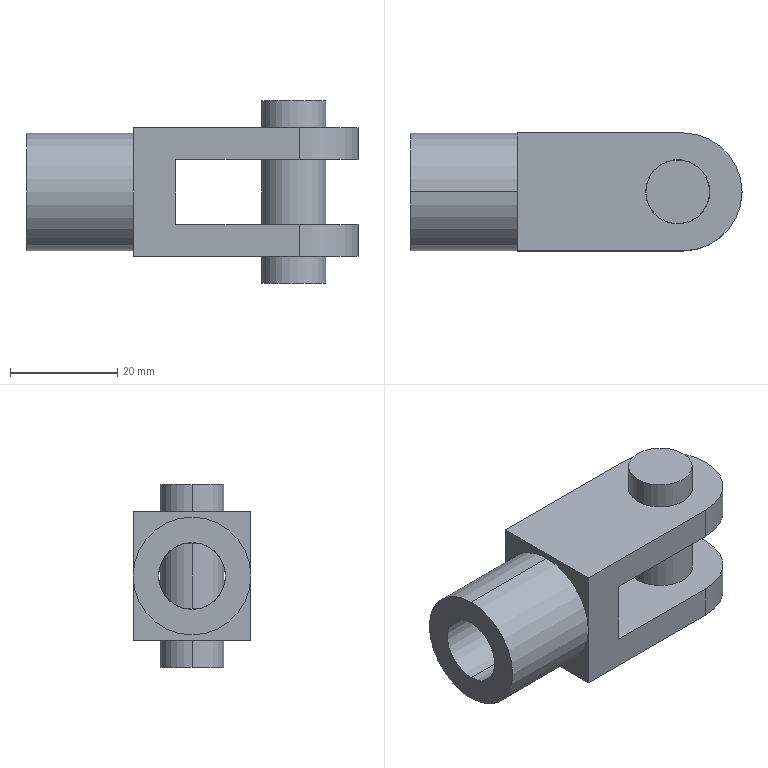Part | SolidWorks | features ICE 4, Extrusion 1, Fillet 1, HoleWzd 1 | 2 solids | 30 faces | box 62 x 22 x 34 mm | volume 19162 mm3 | cylinder 14 | plane 13 | cone 3 | commonest cylinder face diameters 22 x6 12 x4 11.9 x2 12.5 x2
STEP:
#1=CARTESIAN_POINT('',(-11.,11.,12.));
#2=VERTEX_POINT('',#1);
#3=CARTESIAN_POINT('',(-11.,0.,1.));
#4=VERTEX_POINT('',#3);
#5=CARTESIAN_POINT('',(-11.,0.,12.));
#6=DIRECTION('',(-1.,0.,0.));
#7=DIRECTION('',(0.,0.,1.));
#8=AXIS2_PLACEMENT_3D('',#5,#6,#7);
#9=CIRCLE('',#8,11.);
#10=EDGE_CURVE('',#2,#4,#9,.T.);
#11=ORIENTED_EDGE('',*,*,#10,.T.);
#12=CARTESIAN_POINT('',(-31.,0.,1.));
#13=VERTEX_POINT('',#12);
#14=CARTESIAN_POINT('',(-11.,0.,1.));
#15=DIRECTION('',(-1.,0.,0.));
#16=VECTOR('',#15,1000.);
#17=LINE('',#14,#16);
#18=EDGE_CURVE('',#4,#13,#17,.T.);
#19=ORIENTED_EDGE('',*,*,#18,.T.);
#20=CARTESIAN_POINT('',(-31.,0.,23.));
#21=VERTEX_POINT('',#20);
#22=CARTESIAN_POINT('',(-31.,0.,12.));
#23=DIRECTION('',(-1.,0.,0.));
#24=DIRECTION('',(0.,0.,1.));
#25=AXIS2_PLACEMENT_3D('',#22,#23,#24);
#26=CIRCLE('',#25,11.);
#27=EDGE_CURVE('',#21,#13,#26,.T.);
#28=ORIENTED_EDGE('',*,*,#27,.F.);
#29=CARTESIAN_POINT('',(-11.,0.,23.));
#30=VERTEX_POINT('',#29);
#31=CARTESIAN_POINT('',(-11.,0.,23.));
#32=DIRECTION('',(-1.,0.,0.));
#33=VECTOR('',#32,1000.);
#34=LINE('',#31,#33);
#35=EDGE_CURVE('',#30,#21,#34,.T.);
#36=ORIENTED_EDGE('',*,*,#35,.F.);
#37=CARTESIAN_POINT('',(-11.,0.,12.));
#38=DIRECTION('',(-1.,0.,0.));
#39=DIRECTION('',(0.,0.,1.));
#40=AXIS2_PLACEMENT_3D('',#37,#38,#39);
#41=CIRCLE('',#40,11.);
#42=EDGE_CURVE('',#30,#2,#41,.T.);
#43=ORIENTED_EDGE('',*,*,#42,.T.);
#44=EDGE_LOOP('',(#11,#19,#28,#36,#43));
#45=FACE_OUTER_BOUND('',#44,.T.);
#46=CARTESIAN_POINT('',(-11.,0.,12.));
#47=DIRECTION('',(-1.,0.,0.));
#48=DIRECTION('',(0.,0.,1.));
#49=AXIS2_PLACEMENT_3D('',#46,#47,#48);
#50=CYLINDRICAL_SURFACE('',#49,11.);
#51=ADVANCED_FACE('',(#45),#50,.T.);
#52=CARTESIAN_POINT('',(1.65,0.,18.));
#53=VERTEX_POINT('',#52);
#54=CARTESIAN_POINT('',(1.5,1.75,18.));
#55=VERTEX_POINT('',#54);
#56=CARTESIAN_POINT('',(1.65,0.,18.));
#57=CARTESIAN_POINT('',(1.65,0.2911,18.));
#58=CARTESIAN_POINT('',(1.637,0.5828,18.));
#59=CARTESIAN_POINT('',(1.587,1.167,18.));
#60=CARTESIAN_POINT('',(1.549,1.461,18.));
#61=CARTESIAN_POINT('',(1.5,1.75,18.));
#62=B_SPLINE_CURVE_WITH_KNOTS('',3,(#56,#57,#58,#59,#60,#61),.UNSPECIFIED.,.F.,.F.,(4,2,4),(0.03348,0.03433,0.03518),.UNSPECIFIED.);
#63=EDGE_CURVE('',#53,#55,#62,.T.);
#64=ORIENTED_EDGE('',*,*,#63,.F.);
#65=CARTESIAN_POINT('',(1.5,0.,18.25));
#66=VERTEX_POINT('',#65);
#67=CARTESIAN_POINT('',(1.5,0.,18.25));
#68=DIRECTION('',(-0.515,0.,0.8572));
#69=VECTOR('',#68,1000.);
#70=LINE('',#67,#69);
#71=EDGE_CURVE('',#53,#66,#70,.T.);
#72=ORIENTED_EDGE('',*,*,#71,.T.);
#73=CARTESIAN_POINT('',(1.5,0.,12.));
#74=DIRECTION('',(-1.,0.,0.));
#75=DIRECTION('',(0.,0.,1.));
#76=AXIS2_PLACEMENT_3D('',#73,#74,#75);
#77=CIRCLE('',#76,6.25);
#78=EDGE_CURVE('',#66,#55,#77,.T.);
#79=ORIENTED_EDGE('',*,*,#78,.T.);
#80=EDGE_LOOP('',(#64,#72,#79));
#81=FACE_OUTER_BOUND('',#80,.T.);
#82=CARTESIAN_POINT('',(1.5,0.,12.));
#83=DIRECTION('',(-1.,0.,0.));
#84=DIRECTION('',(0.,0.,1.));
#85=AXIS2_PLACEMENT_3D('',#82,#83,#84);
#86=CONICAL_SURFACE('',#85,6.25,1.03);
#87=ADVANCED_FACE('',(#81),#86,.F.);
#88=CARTESIAN_POINT('',(1.5,0.,5.75));
#89=VERTEX_POINT('',#88);
#90=CARTESIAN_POINT('',(1.5,-1.75,6.));
#91=VERTEX_POINT('',#90);
#92=CARTESIAN_POINT('',(1.5,0.,12.));
#93=DIRECTION('',(-1.,0.,0.));
#94=DIRECTION('',(0.,0.,1.));
#95=AXIS2_PLACEMENT_3D('',#92,#93,#94);
#96=CIRCLE('',#95,6.25);
#97=EDGE_CURVE('',#89,#91,#96,.T.);
#98=ORIENTED_EDGE('',*,*,#97,.F.);
#99=CARTESIAN_POINT('',(-31.,0.,5.75));
#100=VERTEX_POINT('',#99);
#101=CARTESIAN_POINT('',(-31.,0.,5.75));
#102=DIRECTION('',(-1.,0.,0.));
#103=VECTOR('',#102,1000.);
#104=LINE('',#101,#103);
#105=EDGE_CURVE('',#89,#100,#104,.T.);
#106=ORIENTED_EDGE('',*,*,#105,.T.);
#107=CARTESIAN_POINT('',(-31.,0.,18.25));
#108=VERTEX_POINT('',#107);
#109=CARTESIAN_POINT('',(-31.,0.,12.));
#110=DIRECTION('',(-1.,0.,0.));
#111=DIRECTION('',(0.,0.,1.));
#112=AXIS2_PLACEMENT_3D('',#109,#110,#111);
#113=CIRCLE('',#112,6.25);
#114=EDGE_CURVE('',#100,#108,#113,.T.);
#115=ORIENTED_EDGE('',*,*,#114,.T.);
#116=CARTESIAN_POINT('',(-31.,0.,18.25));
#117=DIRECTION('',(-1.,0.,0.));
#118=VECTOR('',#117,1000.);
#119=LINE('',#116,#118);
#120=EDGE_CURVE('',#66,#108,#119,.T.);
#121=ORIENTED_EDGE('',*,*,#120,.F.);
#122=CARTESIAN_POINT('',(1.5,-1.75,18.));
#123=VERTEX_POINT('',#122);
#124=CARTESIAN_POINT('',(1.5,0.,12.));
#125=DIRECTION('',(-1.,0.,0.));
#126=DIRECTION('',(0.,0.,1.));
#127=AXIS2_PLACEMENT_3D('',#124,#125,#126);
#128=CIRCLE('',#127,6.25);
#129=EDGE_CURVE('',#123,#66,#128,.T.);
#130=ORIENTED_EDGE('',*,*,#129,.F.);
#131=CARTESIAN_POINT('',(-3.,-1.75,18.));
#132=VERTEX_POINT('',#131);
#133=CARTESIAN_POINT('',(-31.,-1.75,18.));
#134=DIRECTION('',(1.,0.,0.));
#135=VECTOR('',#134,1000.);
#136=LINE('',#133,#135);
#137=EDGE_CURVE('',#132,#123,#136,.T.);
#138=ORIENTED_EDGE('',*,*,#137,.F.);
#139=CARTESIAN_POINT('',(-3.,-1.75,6.));
#140=VERTEX_POINT('',#139);
#141=CARTESIAN_POINT('',(-3.,0.,12.));
#142=DIRECTION('',(-1.,0.,0.));
#143=DIRECTION('',(0.,0.,1.));
#144=AXIS2_PLACEMENT_3D('',#141,#142,#143);
#145=CIRCLE('',#144,6.25);
#146=EDGE_CURVE('',#140,#132,#145,.T.);
#147=ORIENTED_EDGE('',*,*,#146,.F.);
#148=CARTESIAN_POINT('',(-31.,-1.75,6.));
#149=DIRECTION('',(-1.,0.,0.));
#150=VECTOR('',#149,1000.);
#151=LINE('',#148,#150);
#152=EDGE_CURVE('',#91,#140,#151,.T.);
#153=ORIENTED_EDGE('',*,*,#152,.F.);
#154=EDGE_LOOP('',(#98,#106,#115,#121,#130,#138,#147,#153));
#155=FACE_OUTER_BOUND('',#154,.T.);
#156=CARTESIAN_POINT('',(-31.,0.,12.));
#157=DIRECTION('',(-1.,0.,0.));
#158=DIRECTION('',(0.,0.,1.));
#159=AXIS2_PLACEMENT_3D('',#156,#157,#158);
#160=CYLINDRICAL_SURFACE('',#159,6.25);
#161=ADVANCED_FACE('',(#155),#160,.F.);
#162=CARTESIAN_POINT('',(13.,0.,0.));
#163=VERTEX_POINT('',#162);
#164=CARTESIAN_POINT('',(25.,0.,0.));
#165=VERTEX_POINT('',#164);
#166=CARTESIAN_POINT('',(19.,0.,0.));
#167=DIRECTION('',(0.,0.,1.));
#168=DIRECTION('',(1.,0.,0.));
#169=AXIS2_PLACEMENT_3D('',#166,#167,#168);
#170=CIRCLE('',#169,6.);
#171=EDGE_CURVE('',#163,#165,#170,.T.);
#172=ORIENTED_EDGE('',*,*,#171,.F.);
#173=CARTESIAN_POINT('',(13.,0.,6.));
#174=VERTEX_POINT('',#173);
#175=CARTESIAN_POINT('',(13.,0.,0.));
#176=DIRECTION('',(0.,0.,1.));
#177=VECTOR('',#176,1000.);
#178=LINE('',#175,#177);
#179=EDGE_CURVE('',#163,#174,#178,.T.);
#180=ORIENTED_EDGE('',*,*,#179,.T.);
#181=CARTESIAN_POINT('',(25.,0.,6.));
#182=VERTEX_POINT('',#181);
#183=CARTESIAN_POINT('',(19.,0.,6.));
#184=DIRECTION('',(0.,0.,1.));
#185=DIRECTION('',(-1.,0.,0.));
#186=AXIS2_PLACEMENT_3D('',#183,#184,#185);
#187=CIRCLE('',#186,6.);
#188=EDGE_CURVE('',#174,#182,#187,.T.);
#189=ORIENTED_EDGE('',*,*,#188,.T.);
#190=CARTESIAN_POINT('',(25.,0.,0.));
#191=DIRECTION('',(0.,0.,1.));
#192=VECTOR('',#191,1000.);
#193=LINE('',#190,#192);
#194=EDGE_CURVE('',#165,#182,#193,.T.);
#195=ORIENTED_EDGE('',*,*,#194,.F.);
#196=EDGE_LOOP('',(#172,#180,#189,#195));
#197=FACE_OUTER_BOUND('',#196,.T.);
#198=CARTESIAN_POINT('',(19.,0.,0.));
#199=DIRECTION('',(0.,0.,1.));
#200=DIRECTION('',(1.,0.,0.));
#201=AXIS2_PLACEMENT_3D('',#198,#199,#200);
#202=CYLINDRICAL_SURFACE('',#201,6.);
#203=ADVANCED_FACE('',(#197),#202,.F.);
#204=CARTESIAN_POINT('',(25.,0.,18.));
#205=VERTEX_POINT('',#204);
#206=CARTESIAN_POINT('',(13.,0.,18.));
#207=VERTEX_POINT('',#206);
#208=CARTESIAN_POINT('',(19.,0.,18.));
#209=DIRECTION('',(0.,0.,-1.));
#210=DIRECTION('',(1.,0.,0.));
#211=AXIS2_PLACEMENT_3D('',#208,#209,#210);
#212=CIRCLE('',#211,6.);
#213=EDGE_CURVE('',#205,#207,#212,.T.);
#214=ORIENTED_EDGE('',*,*,#213,.T.);
#215=CARTESIAN_POINT('',(13.,0.,24.));
#216=VERTEX_POINT('',#215);
#217=CARTESIAN_POINT('',(13.,0.,0.));
#218=DIRECTION('',(0.,0.,1.));
#219=VECTOR('',#218,1000.);
#220=LINE('',#217,#219);
#221=EDGE_CURVE('',#207,#216,#220,.T.);
#222=ORIENTED_EDGE('',*,*,#221,.T.);
#223=CARTESIAN_POINT('',(25.,0.,24.));
#224=VERTEX_POINT('',#223);
#225=CARTESIAN_POINT('',(19.,0.,24.));
#226=DIRECTION('',(0.,0.,1.));
#227=DIRECTION('',(1.,0.,0.));
#228=AXIS2_PLACEMENT_3D('',#225,#226,#227);
#229=CIRCLE('',#228,6.);
#230=EDGE_CURVE('',#216,#224,#229,.T.);
#231=ORIENTED_EDGE('',*,*,#230,.T.);
#232=CARTESIAN_POINT('',(25.,0.,0.));
#233=DIRECTION('',(0.,0.,1.));
#234=VECTOR('',#233,1000.);
#235=LINE('',#232,#234);
#236=EDGE_CURVE('',#205,#224,#235,.T.);
#237=ORIENTED_EDGE('',*,*,#236,.F.);
#238=EDGE_LOOP('',(#214,#222,#231,#237));
#239=FACE_OUTER_BOUND('',#238,.T.);
#240=CARTESIAN_POINT('',(19.,0.,0.));
#241=DIRECTION('',(0.,0.,1.));
#242=DIRECTION('',(1.,0.,0.));
#243=AXIS2_PLACEMENT_3D('',#240,#241,#242);
#244=CYLINDRICAL_SURFACE('',#243,6.);
#245=ADVANCED_FACE('',(#239),#244,.F.);
#246=CARTESIAN_POINT('',(20.,11.,6.));
#247=VERTEX_POINT('',#246);
#248=CARTESIAN_POINT('',(-3.,11.,6.));
#249=VERTEX_POINT('',#248);
#250=CARTESIAN_POINT('',(31.,11.,6.));
#251=DIRECTION('',(-1.,0.,0.));
#252=VECTOR('',#251,1000.);
#253=LINE('',#250,#252);
#254=EDGE_CURVE('',#247,#249,#253,.T.);
#255=ORIENTED_EDGE('',*,*,#254,.F.);
#256=CARTESIAN_POINT('',(20.,11.,0.));
#257=VERTEX_POINT('',#256);
#258=CARTESIAN_POINT('',(20.,11.,24.));
#259=DIRECTION('',(0.,0.,-1.));
#260=VECTOR('',#259,1000.);
#261=LINE('',#258,#260);
#262=EDGE_CURVE('',#247,#257,#261,.T.);
#263=ORIENTED_EDGE('',*,*,#262,.T.);
#264=CARTESIAN_POINT('',(-11.,11.,0.));
#265=VERTEX_POINT('',#264);
#266=CARTESIAN_POINT('',(-31.,11.,0.));
#267=DIRECTION('',(-1.,0.,0.));
#268=VECTOR('',#267,1000.);
#269=LINE('',#266,#268);
#270=EDGE_CURVE('',#257,#265,#269,.T.);
#271=ORIENTED_EDGE('',*,*,#270,.T.);
#272=CARTESIAN_POINT('',(-11.,11.,24.));
#273=DIRECTION('',(0.,0.,-1.));
#274=VECTOR('',#273,1000.);
#275=LINE('',#272,#274);
#276=EDGE_CURVE('',#2,#265,#275,.T.);
#277=ORIENTED_EDGE('',*,*,#276,.F.);
#278=CARTESIAN_POINT('',(-11.,11.,24.));
#279=VERTEX_POINT('',#278);
#280=CARTESIAN_POINT('',(-11.,11.,24.));
#281=DIRECTION('',(0.,0.,-1.));
#282=VECTOR('',#281,1000.);
#283=LINE('',#280,#282);
#284=EDGE_CURVE('',#279,#2,#283,.T.);
#285=ORIENTED_EDGE('',*,*,#284,.F.);
#286=CARTESIAN_POINT('',(20.,11.,24.));
#287=VERTEX_POINT('',#286);
#288=CARTESIAN_POINT('',(-31.,11.,24.));
#289=DIRECTION('',(-1.,0.,0.));
#290=VECTOR('',#289,1000.);
#291=LINE('',#288,#290);
#292=EDGE_CURVE('',#287,#279,#291,.T.);
#293=ORIENTED_EDGE('',*,*,#292,.F.);
#294=CARTESIAN_POINT('',(20.,11.,18.));
#295=VERTEX_POINT('',#294);
#296=CARTESIAN_POINT('',(20.,11.,24.));
#297=DIRECTION('',(0.,0.,-1.));
#298=VECTOR('',#297,1000.);
#299=LINE('',#296,#298);
#300=EDGE_CURVE('',#287,#295,#299,.T.);
#301=ORIENTED_EDGE('',*,*,#300,.T.);
#302=CARTESIAN_POINT('',(-3.,11.,18.));
#303=VERTEX_POINT('',#302);
#304=CARTESIAN_POINT('',(31.,11.,18.));
#305=DIRECTION('',(1.,0.,0.));
#306=VECTOR('',#305,1000.);
#307=LINE('',#304,#306);
#308=EDGE_CURVE('',#303,#295,#307,.T.);
#309=ORIENTED_EDGE('',*,*,#308,.F.);
#310=CARTESIAN_POINT('',(-3.,11.,6.));
#311=DIRECTION('',(0.,0.,1.));
#312=VECTOR('',#311,1000.);
#313=LINE('',#310,#312);
#314=EDGE_CURVE('',#249,#303,#313,.T.);
#315=ORIENTED_EDGE('',*,*,#314,.F.);
#316=EDGE_LOOP('',(#255,#263,#271,#277,#285,#293,#301,#309,#315));
#317=FACE_OUTER_BOUND('',#316,.T.);
#318=CARTESIAN_POINT('',(-31.,11.,24.));
#319=DIRECTION('',(0.,-1.,0.));
#320=DIRECTION('',(0.,0.,-1.));
#321=AXIS2_PLACEMENT_3D('',#318,#319,#320);
#322=PLANE('',#321);
#323=ADVANCED_FACE('',(#317),#322,.F.);
#324=CARTESIAN_POINT('',(-31.,0.,12.));
#325=DIRECTION('',(-1.,0.,0.));
#326=DIRECTION('',(0.,0.,1.));
#327=AXIS2_PLACEMENT_3D('',#324,#325,#326);
#328=CIRCLE('',#327,6.25);
#329=EDGE_CURVE('',#108,#100,#328,.T.);
#330=ORIENTED_EDGE('',*,*,#329,.F.);
#331=ORIENTED_EDGE('',*,*,#114,.F.);
#332=EDGE_LOOP('',(#330,#331));
#333=FACE_BOUND('',#332,.T.);
#334=ORIENTED_EDGE('',*,*,#27,.T.);
#335=CARTESIAN_POINT('',(-31.,0.,12.));
#336=DIRECTION('',(-1.,0.,0.));
#337=DIRECTION('',(0.,0.,1.));
#338=AXIS2_PLACEMENT_3D('',#335,#336,#337);
#339=CIRCLE('',#338,11.);
#340=EDGE_CURVE('',#13,#21,#339,.T.);
#341=ORIENTED_EDGE('',*,*,#340,.T.);
#342=EDGE_LOOP('',(#334,#341));
#343=FACE_OUTER_BOUND('',#342,.T.);
#344=CARTESIAN_POINT('',(-31.,11.,24.));
#345=DIRECTION('',(1.,0.,0.));
#346=DIRECTION('',(0.,1.,0.));
#347=AXIS2_PLACEMENT_3D('',#344,#345,#346);
#348=PLANE('',#347);
#349=ADVANCED_FACE('',(#333,#343),#348,.F.);
#350=CARTESIAN_POINT('',(-11.,-11.,0.));
#351=VERTEX_POINT('',#350);
#352=CARTESIAN_POINT('',(20.,-11.,0.));
#353=VERTEX_POINT('',#352);
#354=CARTESIAN_POINT('',(-31.,-11.,0.));
#355=DIRECTION('',(1.,0.,0.));
#356=VECTOR('',#355,1000.);
#357=LINE('',#354,#356);
#358=EDGE_CURVE('',#351,#353,#357,.T.);
#359=ORIENTED_EDGE('',*,*,#358,.T.);
#360=CARTESIAN_POINT('',(20.,-11.,6.));
#361=VERTEX_POINT('',#360);
#362=CARTESIAN_POINT('',(20.,-11.,24.));
#363=DIRECTION('',(0.,0.,1.));
#364=VECTOR('',#363,1000.);
#365=LINE('',#362,#364);
#366=EDGE_CURVE('',#353,#361,#365,.T.);
#367=ORIENTED_EDGE('',*,*,#366,.T.);
#368=CARTESIAN_POINT('',(-3.,-11.,6.));
#369=VERTEX_POINT('',#368);
#370=CARTESIAN_POINT('',(31.,-11.,6.));
#371=DIRECTION('',(-1.,0.,0.));
#372=VECTOR('',#371,1000.);
#373=LINE('',#370,#372);
#374=EDGE_CURVE('',#361,#369,#373,.T.);
#375=ORIENTED_EDGE('',*,*,#374,.T.);
#376=CARTESIAN_POINT('',(-3.,-11.,18.));
#377=VERTEX_POINT('',#376);
#378=CARTESIAN_POINT('',(-3.,-11.,6.));
#379=DIRECTION('',(0.,0.,1.));
#380=VECTOR('',#379,1000.);
#381=LINE('',#378,#380);
#382=EDGE_CURVE('',#369,#377,#381,.T.);
#383=ORIENTED_EDGE('',*,*,#382,.T.);
#384=CARTESIAN_POINT('',(20.,-11.,18.));
#385=VERTEX_POINT('',#384);
#386=CARTESIAN_POINT('',(31.,-11.,18.));
#387=DIRECTION('',(1.,0.,0.));
#388=VECTOR('',#387,1000.);
#389=LINE('',#386,#388);
#390=EDGE_CURVE('',#377,#385,#389,.T.);
#391=ORIENTED_EDGE('',*,*,#390,.T.);
#392=CARTESIAN_POINT('',(20.,-11.,24.));
#393=VERTEX_POINT('',#392);
#394=CARTESIAN_POINT('',(20.,-11.,24.));
#395=DIRECTION('',(0.,0.,1.));
#396=VECTOR('',#395,1000.);
#397=LINE('',#394,#396);
#398=EDGE_CURVE('',#385,#393,#397,.T.);
#399=ORIENTED_EDGE('',*,*,#398,.T.);
#400=CARTESIAN_POINT('',(-11.,-11.,24.));
#401=VERTEX_POINT('',#400);
#402=CARTESIAN_POINT('',(-31.,-11.,24.));
#403=DIRECTION('',(1.,0.,0.));
#404=VECTOR('',#403,1000.);
#405=LINE('',#402,#404);
#406=EDGE_CURVE('',#401,#393,#405,.T.);
#407=ORIENTED_EDGE('',*,*,#406,.F.);
#408=CARTESIAN_POINT('',(-11.,-11.,12.));
#409=VERTEX_POINT('',#408);
#410=CARTESIAN_POINT('',(-11.,-11.,24.));
#411=DIRECTION('',(0.,0.,1.));
#412=VECTOR('',#411,1000.);
#413=LINE('',#410,#412);
#414=EDGE_CURVE('',#409,#401,#413,.T.);
#415=ORIENTED_EDGE('',*,*,#414,.F.);
#416=CARTESIAN_POINT('',(-11.,-11.,24.));
#417=DIRECTION('',(0.,0.,1.));
#418=VECTOR('',#417,1000.);
#419=LINE('',#416,#418);
#420=EDGE_CURVE('',#351,#409,#419,.T.);
#421=ORIENTED_EDGE('',*,*,#420,.F.);
#422=EDGE_LOOP('',(#359,#367,#375,#383,#391,#399,#407,#415,#421));
#423=FACE_OUTER_BOUND('',#422,.T.);
#424=CARTESIAN_POINT('',(-31.,-11.,24.));
#425=DIRECTION('',(0.,1.,0.));
#426=DIRECTION('',(0.,0.,1.));
#427=AXIS2_PLACEMENT_3D('',#424,#425,#426);
#428=PLANE('',#427);
#429=ADVANCED_FACE('',(#423),#428,.F.);
#430=CARTESIAN_POINT('',(19.,0.,24.));
#431=DIRECTION('',(0.,0.,1.));
#432=DIRECTION('',(1.,0.,0.));
#433=AXIS2_PLACEMENT_3D('',#430,#431,#432);
#434=CIRCLE('',#433,6.);
#435=EDGE_CURVE('',#224,#216,#434,.T.);
#436=ORIENTED_EDGE('',*,*,#435,.F.);
#437=ORIENTED_EDGE('',*,*,#230,.F.);
#438=EDGE_LOOP('',(#436,#437));
#439=FACE_BOUND('',#438,.T.);
#440=ORIENTED_EDGE('',*,*,#406,.T.);
#441=CARTESIAN_POINT('',(31.,0.,24.));
#442=VERTEX_POINT('',#441);
#443=CARTESIAN_POINT('',(20.,0.,24.));
#444=DIRECTION('',(0.,0.,1.));
#445=DIRECTION('',(1.,0.,0.));
#446=AXIS2_PLACEMENT_3D('',#443,#444,#445);
#447=CIRCLE('',#446,11.);
#448=EDGE_CURVE('',#393,#442,#447,.T.);
#449=ORIENTED_EDGE('',*,*,#448,.T.);
#450=CARTESIAN_POINT('',(20.,0.,24.));
#451=DIRECTION('',(0.,0.,1.));
#452=DIRECTION('',(1.,0.,0.));
#453=AXIS2_PLACEMENT_3D('',#450,#451,#452);
#454=CIRCLE('',#453,11.);
#455=EDGE_CURVE('',#442,#287,#454,.T.);
#456=ORIENTED_EDGE('',*,*,#455,.T.);
#457=ORIENTED_EDGE('',*,*,#292,.T.);
#458=CARTESIAN_POINT('',(-11.,0.,24.));
#459=DIRECTION('',(0.,-1.,0.));
#460=VECTOR('',#459,1000.);
#461=LINE('',#458,#460);
#462=EDGE_CURVE('',#279,#401,#461,.T.);
#463=ORIENTED_EDGE('',*,*,#462,.T.);
#464=EDGE_LOOP('',(#440,#449,#456,#457,#463));
#465=FACE_OUTER_BOUND('',#464,.T.);
#466=CARTESIAN_POINT('',(0.,0.,24.));
#467=DIRECTION('',(0.,0.,1.));
#468=DIRECTION('',(1.,0.,0.));
#469=AXIS2_PLACEMENT_3D('',#466,#467,#468);
#470=PLANE('',#469);
#471=ADVANCED_FACE('',(#439,#465),#470,.T.);
#472=CARTESIAN_POINT('',(19.,0.,0.));
#473=DIRECTION('',(0.,0.,1.));
#474=DIRECTION('',(1.,0.,0.));
#475=AXIS2_PLACEMENT_3D('',#472,#473,#474);
#476=CIRCLE('',#475,6.);
#477=EDGE_CURVE('',#165,#163,#476,.T.);
#478=ORIENTED_EDGE('',*,*,#477,.T.);
#479=ORIENTED_EDGE('',*,*,#171,.T.);
#480=EDGE_LOOP('',(#478,#479));
#481=FACE_BOUND('',#480,.T.);
#482=CARTESIAN_POINT('',(31.,0.,0.));
#483=VERTEX_POINT('',#482);
#484=CARTESIAN_POINT('',(20.,0.,0.));
#485=DIRECTION('',(0.,0.,-1.));
#486=DIRECTION('',(1.,0.,0.));
#487=AXIS2_PLACEMENT_3D('',#484,#485,#486);
#488=CIRCLE('',#487,11.);
#489=EDGE_CURVE('',#257,#483,#488,.T.);
#490=ORIENTED_EDGE('',*,*,#489,.T.);
#491=CARTESIAN_POINT('',(20.,0.,0.));
#492=DIRECTION('',(0.,0.,-1.));
#493=DIRECTION('',(1.,0.,0.));
#494=AXIS2_PLACEMENT_3D('',#491,#492,#493);
#495=CIRCLE('',#494,11.);
#496=EDGE_CURVE('',#483,#353,#495,.T.);
#497=ORIENTED_EDGE('',*,*,#496,.T.);
#498=ORIENTED_EDGE('',*,*,#358,.F.);
#499=CARTESIAN_POINT('',(-11.,0.,0.));
#500=DIRECTION('',(0.,-1.,0.));
#501=VECTOR('',#500,1000.);
#502=LINE('',#499,#501);
#503=EDGE_CURVE('',#265,#351,#502,.T.);
#504=ORIENTED_EDGE('',*,*,#503,.F.);
#505=ORIENTED_EDGE('',*,*,#270,.F.);
#506=EDGE_LOOP('',(#490,#497,#498,#504,#505));
#507=FACE_OUTER_BOUND('',#506,.T.);
#508=CARTESIAN_POINT('',(0.,0.,0.));
#509=DIRECTION('',(0.,0.,1.));
#510=DIRECTION('',(1.,0.,0.));
#511=AXIS2_PLACEMENT_3D('',#508,#509,#510);
#512=PLANE('',#511);
#513=ADVANCED_FACE('',(#481,#507),#512,.F.);
#514=CARTESIAN_POINT('',(-3.,1.75,18.));
#515=VERTEX_POINT('',#514);
#516=CARTESIAN_POINT('',(-3.,-11.,18.));
#517=DIRECTION('',(0.,1.,0.));
#518=VECTOR('',#517,1000.);
#519=LINE('',#516,#518);
#520=EDGE_CURVE('',#515,#303,#519,.T.);
#521=ORIENTED_EDGE('',*,*,#520,.F.);
#522=CARTESIAN_POINT('',(-3.,1.75,6.));
#523=VERTEX_POINT('',#522);
#524=CARTESIAN_POINT('',(-3.,0.,12.));
#525=DIRECTION('',(-1.,0.,0.));
#526=DIRECTION('',(0.,0.,1.));
#527=AXIS2_PLACEMENT_3D('',#524,#525,#526);
#528=CIRCLE('',#527,6.25);
#529=EDGE_CURVE('',#515,#523,#528,.T.);
#530=ORIENTED_EDGE('',*,*,#529,.T.);
#531=CARTESIAN_POINT('',(-3.,-11.,6.));
#532=DIRECTION('',(0.,1.,0.));
#533=VECTOR('',#532,1000.);
#534=LINE('',#531,#533);
#535=EDGE_CURVE('',#523,#249,#534,.T.);
#536=ORIENTED_EDGE('',*,*,#535,.T.);
#537=ORIENTED_EDGE('',*,*,#314,.T.);
#538=EDGE_LOOP('',(#521,#530,#536,#537));
#539=FACE_OUTER_BOUND('',#538,.T.);
#540=CARTESIAN_POINT('',(-3.,-11.,6.));
#541=DIRECTION('',(-1.,0.,0.));
#542=DIRECTION('',(0.,0.,1.));
#543=AXIS2_PLACEMENT_3D('',#540,#541,#542);
#544=PLANE('',#543);
#545=ADVANCED_FACE('',(#539),#544,.F.);
#546=ORIENTED_EDGE('',*,*,#221,.F.);
#547=CARTESIAN_POINT('',(19.,0.,18.));
#548=DIRECTION('',(0.,0.,-1.));
#549=DIRECTION('',(1.,0.,0.));
#550=AXIS2_PLACEMENT_3D('',#547,#548,#549);
#551=CIRCLE('',#550,6.);
#552=EDGE_CURVE('',#207,#205,#551,.T.);
#553=ORIENTED_EDGE('',*,*,#552,.T.);
#554=ORIENTED_EDGE('',*,*,#236,.T.);
#555=ORIENTED_EDGE('',*,*,#435,.T.);
#556=EDGE_LOOP('',(#546,#553,#554,#555));
#557=FACE_OUTER_BOUND('',#556,.T.);
#558=CARTESIAN_POINT('',(19.,0.,0.));
#559=DIRECTION('',(0.,0.,1.));
#560=DIRECTION('',(1.,0.,0.));
#561=AXIS2_PLACEMENT_3D('',#558,#559,#560);
#562=CYLINDRICAL_SURFACE('',#561,6.);
#563=ADVANCED_FACE('',(#557),#562,.F.);
#564=ORIENTED_EDGE('',*,*,#179,.F.);
#565=ORIENTED_EDGE('',*,*,#477,.F.);
#566=ORIENTED_EDGE('',*,*,#194,.T.);
#567=CARTESIAN_POINT('',(19.,0.,6.));
#568=DIRECTION('',(0.,0.,1.));
#569=DIRECTION('',(-1.,0.,0.));
#570=AXIS2_PLACEMENT_3D('',#567,#568,#569);
#571=CIRCLE('',#570,6.);
#572=EDGE_CURVE('',#182,#174,#571,.T.);
#573=ORIENTED_EDGE('',*,*,#572,.T.);
#574=EDGE_LOOP('',(#564,#565,#566,#573));
#575=FACE_OUTER_BOUND('',#574,.T.);
#576=CARTESIAN_POINT('',(19.,0.,0.));
#577=DIRECTION('',(0.,0.,1.));
#578=DIRECTION('',(1.,0.,0.));
#579=AXIS2_PLACEMENT_3D('',#576,#577,#578);
#580=CYLINDRICAL_SURFACE('',#579,6.);
#581=ADVANCED_FACE('',(#575),#580,.F.);
#582=CARTESIAN_POINT('',(31.,0.,18.));
#583=VERTEX_POINT('',#582);
#584=CARTESIAN_POINT('',(20.,0.,18.));
#585=DIRECTION('',(0.,0.,-1.));
#586=DIRECTION('',(1.,0.,0.));
#587=AXIS2_PLACEMENT_3D('',#584,#585,#586);
#588=CIRCLE('',#587,11.);
#589=EDGE_CURVE('',#295,#583,#588,.T.);
#590=ORIENTED_EDGE('',*,*,#589,.T.);
#591=CARTESIAN_POINT('',(20.,0.,18.));
#592=DIRECTION('',(0.,0.,-1.));
#593=DIRECTION('',(1.,0.,0.));
#594=AXIS2_PLACEMENT_3D('',#591,#592,#593);
#595=CIRCLE('',#594,11.);
#596=EDGE_CURVE('',#583,#385,#595,.T.);
#597=ORIENTED_EDGE('',*,*,#596,.T.);
#598=ORIENTED_EDGE('',*,*,#390,.F.);
#599=CARTESIAN_POINT('',(-3.,-11.,18.));
#600=DIRECTION('',(0.,1.,0.));
#601=VECTOR('',#600,1000.);
#602=LINE('',#599,#601);
#603=EDGE_CURVE('',#377,#132,#602,.T.);
#604=ORIENTED_EDGE('',*,*,#603,.T.);
#605=ORIENTED_EDGE('',*,*,#137,.T.);
#606=CARTESIAN_POINT('',(1.5,-1.75,18.));
#607=CARTESIAN_POINT('',(1.598,-1.168,18.));
#608=CARTESIAN_POINT('',(1.65,-0.5852,18.));
#609=CARTESIAN_POINT('',(1.65,0.,18.));
#610=B_SPLINE_CURVE_WITH_KNOTS('',3,(#606,#607,#608,#609),.UNSPECIFIED.,.F.,.F.,(4,4),(0.03177,0.03348),.UNSPECIFIED.);
#611=EDGE_CURVE('',#123,#53,#610,.T.);
#612=ORIENTED_EDGE('',*,*,#611,.T.);
#613=ORIENTED_EDGE('',*,*,#63,.T.);
#614=CARTESIAN_POINT('',(-31.,1.75,18.));
#615=DIRECTION('',(-1.,0.,0.));
#616=VECTOR('',#615,1000.);
#617=LINE('',#614,#616);
#618=EDGE_CURVE('',#55,#515,#617,.T.);
#619=ORIENTED_EDGE('',*,*,#618,.T.);
#620=ORIENTED_EDGE('',*,*,#520,.T.);
#621=ORIENTED_EDGE('',*,*,#308,.T.);
#622=EDGE_LOOP('',(#590,#597,#598,#604,#605,#612,#613,#619,#620,#621));
#623=FACE_OUTER_BOUND('',#622,.T.);
#624=ORIENTED_EDGE('',*,*,#213,.F.);
#625=ORIENTED_EDGE('',*,*,#552,.F.);
#626=EDGE_LOOP('',(#624,#625));
#627=FACE_BOUND('',#626,.T.);
#628=CARTESIAN_POINT('',(31.,-11.,18.));
#629=DIRECTION('',(0.,0.,1.));
#630=DIRECTION('',(1.,0.,0.));
#631=AXIS2_PLACEMENT_3D('',#628,#629,#630);
#632=PLANE('',#631);
#633=ADVANCED_FACE('',(#623,#627),#632,.F.);
#634=ORIENTED_EDGE('',*,*,#374,.F.);
#635=CARTESIAN_POINT('',(31.,0.,6.));
#636=VERTEX_POINT('',#635);
#637=CARTESIAN_POINT('',(20.,0.,6.));
#638=DIRECTION('',(0.,0.,1.));
#639=DIRECTION('',(-1.,0.,0.));
#640=AXIS2_PLACEMENT_3D('',#637,#638,#639);
#641=CIRCLE('',#640,11.);
#642=EDGE_CURVE('',#361,#636,#641,.T.);
#643=ORIENTED_EDGE('',*,*,#642,.T.);
#644=CARTESIAN_POINT('',(20.,0.,6.));
#645=DIRECTION('',(0.,0.,1.));
#646=DIRECTION('',(-1.,0.,0.));
#647=AXIS2_PLACEMENT_3D('',#644,#645,#646);
#648=CIRCLE('',#647,11.);
#649=EDGE_CURVE('',#636,#247,#648,.T.);
#650=ORIENTED_EDGE('',*,*,#649,.T.);
#651=ORIENTED_EDGE('',*,*,#254,.T.);
#652=ORIENTED_EDGE('',*,*,#535,.F.);
#653=CARTESIAN_POINT('',(1.5,1.75,6.));
#654=VERTEX_POINT('',#653);
#655=CARTESIAN_POINT('',(-31.,1.75,6.));
#656=DIRECTION('',(1.,0.,0.));
#657=VECTOR('',#656,1000.);
#658=LINE('',#655,#657);
#659=EDGE_CURVE('',#523,#654,#658,.T.);
#660=ORIENTED_EDGE('',*,*,#659,.T.);
#661=CARTESIAN_POINT('',(1.5,1.75,6.));
#662=CARTESIAN_POINT('',(1.549,1.46,6.));
#663=CARTESIAN_POINT('',(1.587,1.166,6.));
#664=CARTESIAN_POINT('',(1.638,0.5799,6.));
#665=CARTESIAN_POINT('',(1.65,0.2875,6.));
#666=CARTESIAN_POINT('',(1.65,-0.5881,6.));
#667=CARTESIAN_POINT('',(1.598,-1.17,6.));
#668=CARTESIAN_POINT('',(1.5,-1.75,6.));
#669=B_SPLINE_CURVE_WITH_KNOTS('',3,(#661,#662,#663,#664,#665,#666,#667,#668),.UNSPECIFIED.,.F.,.F.,(4,2,2,4),(0.03012,0.031,0.03187,0.03363),.UNSPECIFIED.);
#670=EDGE_CURVE('',#654,#91,#669,.T.);
#671=ORIENTED_EDGE('',*,*,#670,.T.);
#672=ORIENTED_EDGE('',*,*,#152,.T.);
#673=CARTESIAN_POINT('',(-3.,-11.,6.));
#674=DIRECTION('',(0.,1.,0.));
#675=VECTOR('',#674,1000.);
#676=LINE('',#673,#675);
#677=EDGE_CURVE('',#369,#140,#676,.T.);
#678=ORIENTED_EDGE('',*,*,#677,.F.);
#679=EDGE_LOOP('',(#634,#643,#650,#651,#652,#660,#671,#672,#678));
#680=FACE_OUTER_BOUND('',#679,.T.);
#681=ORIENTED_EDGE('',*,*,#572,.F.);
#682=ORIENTED_EDGE('',*,*,#188,.F.);
#683=EDGE_LOOP('',(#681,#682));
#684=FACE_BOUND('',#683,.T.);
#685=CARTESIAN_POINT('',(31.,-11.,6.));
#686=DIRECTION('',(0.,0.,-1.));
#687=DIRECTION('',(-1.,0.,0.));
#688=AXIS2_PLACEMENT_3D('',#685,#686,#687);
#689=PLANE('',#688);
#690=ADVANCED_FACE('',(#680,#684),#689,.F.);
#691=ORIENTED_EDGE('',*,*,#677,.T.);
#692=ORIENTED_EDGE('',*,*,#146,.T.);
#693=ORIENTED_EDGE('',*,*,#603,.F.);
#694=ORIENTED_EDGE('',*,*,#382,.F.);
#695=EDGE_LOOP('',(#691,#692,#693,#694));
#696=FACE_OUTER_BOUND('',#695,.T.);
#697=CARTESIAN_POINT('',(-3.,-11.,6.));
#698=DIRECTION('',(-1.,0.,0.));
#699=DIRECTION('',(0.,0.,1.));
#700=AXIS2_PLACEMENT_3D('',#697,#698,#699);
#701=PLANE('',#700);
#702=ADVANCED_FACE('',(#696),#701,.F.);
#703=ORIENTED_EDGE('',*,*,#105,.F.);
#704=CARTESIAN_POINT('',(1.5,0.,12.));
#705=DIRECTION('',(-1.,0.,0.));
#706=DIRECTION('',(0.,0.,1.));
#707=AXIS2_PLACEMENT_3D('',#704,#705,#706);
#708=CIRCLE('',#707,6.25);
#709=EDGE_CURVE('',#654,#89,#708,.T.);
#710=ORIENTED_EDGE('',*,*,#709,.F.);
#711=ORIENTED_EDGE('',*,*,#659,.F.);
#712=ORIENTED_EDGE('',*,*,#529,.F.);
#713=ORIENTED_EDGE('',*,*,#618,.F.);
#714=ORIENTED_EDGE('',*,*,#78,.F.);
#715=ORIENTED_EDGE('',*,*,#120,.T.);
#716=ORIENTED_EDGE('',*,*,#329,.T.);
#717=EDGE_LOOP('',(#703,#710,#711,#712,#713,#714,#715,#716));
#718=FACE_OUTER_BOUND('',#717,.T.);
#719=CARTESIAN_POINT('',(-31.,0.,12.));
#720=DIRECTION('',(-1.,0.,0.));
#721=DIRECTION('',(0.,0.,1.));
#722=AXIS2_PLACEMENT_3D('',#719,#720,#721);
#723=CYLINDRICAL_SURFACE('',#722,6.25);
#724=ADVANCED_FACE('',(#718),#723,.F.);
#725=ORIENTED_EDGE('',*,*,#71,.F.);
#726=ORIENTED_EDGE('',*,*,#611,.F.);
#727=ORIENTED_EDGE('',*,*,#129,.T.);
#728=EDGE_LOOP('',(#725,#726,#727));
#729=FACE_OUTER_BOUND('',#728,.T.);
#730=CARTESIAN_POINT('',(1.5,0.,12.));
#731=DIRECTION('',(-1.,0.,0.));
#732=DIRECTION('',(0.,0.,1.));
#733=AXIS2_PLACEMENT_3D('',#730,#731,#732);
#734=CONICAL_SURFACE('',#733,6.25,1.03);
#735=ADVANCED_FACE('',(#729),#734,.F.);
#736=ORIENTED_EDGE('',*,*,#709,.T.);
#737=ORIENTED_EDGE('',*,*,#97,.T.);
#738=ORIENTED_EDGE('',*,*,#670,.F.);
#739=EDGE_LOOP('',(#736,#737,#738));
#740=FACE_OUTER_BOUND('',#739,.T.);
#741=CARTESIAN_POINT('',(1.5,0.,12.));
#742=DIRECTION('',(-1.,0.,0.));
#743=DIRECTION('',(0.,0.,1.));
#744=AXIS2_PLACEMENT_3D('',#741,#742,#743);
#745=CONICAL_SURFACE('',#744,6.25,1.03);
#746=ADVANCED_FACE('',(#740),#745,.F.);
#747=ORIENTED_EDGE('',*,*,#18,.F.);
#748=CARTESIAN_POINT('',(-11.,0.,12.));
#749=DIRECTION('',(-1.,0.,0.));
#750=DIRECTION('',(0.,0.,1.));
#751=AXIS2_PLACEMENT_3D('',#748,#749,#750);
#752=CIRCLE('',#751,11.);
#753=EDGE_CURVE('',#4,#409,#752,.T.);
#754=ORIENTED_EDGE('',*,*,#753,.T.);
#755=CARTESIAN_POINT('',(-11.,0.,12.));
#756=DIRECTION('',(-1.,0.,0.));
#757=DIRECTION('',(0.,0.,1.));
#758=AXIS2_PLACEMENT_3D('',#755,#756,#757);
#759=CIRCLE('',#758,11.);
#760=EDGE_CURVE('',#409,#30,#759,.T.);
#761=ORIENTED_EDGE('',*,*,#760,.T.);
#762=ORIENTED_EDGE('',*,*,#35,.T.);
#763=ORIENTED_EDGE('',*,*,#340,.F.);
#764=EDGE_LOOP('',(#747,#754,#761,#762,#763));
#765=FACE_OUTER_BOUND('',#764,.T.);
#766=CARTESIAN_POINT('',(-11.,0.,12.));
#767=DIRECTION('',(-1.,0.,0.));
#768=DIRECTION('',(0.,0.,1.));
#769=AXIS2_PLACEMENT_3D('',#766,#767,#768);
#770=CYLINDRICAL_SURFACE('',#769,11.);
#771=ADVANCED_FACE('',(#765),#770,.T.);
#772=ORIENTED_EDGE('',*,*,#414,.T.);
#773=ORIENTED_EDGE('',*,*,#462,.F.);
#774=ORIENTED_EDGE('',*,*,#284,.T.);
#775=ORIENTED_EDGE('',*,*,#42,.F.);
#776=ORIENTED_EDGE('',*,*,#760,.F.);
#777=EDGE_LOOP('',(#772,#773,#774,#775,#776));
#778=FACE_OUTER_BOUND('',#777,.T.);
#779=CARTESIAN_POINT('',(-11.,0.,12.));
#780=DIRECTION('',(-1.,0.,0.));
#781=DIRECTION('',(0.,0.,1.));
#782=AXIS2_PLACEMENT_3D('',#779,#780,#781);
#783=PLANE('',#782);
#784=ADVANCED_FACE('',(#778),#783,.T.);
#785=ORIENTED_EDGE('',*,*,#276,.T.);
#786=ORIENTED_EDGE('',*,*,#503,.T.);
#787=ORIENTED_EDGE('',*,*,#420,.T.);
#788=ORIENTED_EDGE('',*,*,#753,.F.);
#789=ORIENTED_EDGE('',*,*,#10,.F.);
#790=EDGE_LOOP('',(#785,#786,#787,#788,#789));
#791=FACE_OUTER_BOUND('',#790,.T.);
#792=CARTESIAN_POINT('',(-11.,0.,12.));
#793=DIRECTION('',(-1.,0.,0.));
#794=DIRECTION('',(0.,0.,1.));
#795=AXIS2_PLACEMENT_3D('',#792,#793,#794);
#796=PLANE('',#795);
#797=ADVANCED_FACE('',(#791),#796,.T.);
#798=ORIENTED_EDGE('',*,*,#262,.F.);
#799=ORIENTED_EDGE('',*,*,#649,.F.);
#800=CARTESIAN_POINT('',(31.,0.,24.));
#801=DIRECTION('',(0.,0.,1.));
#802=VECTOR('',#801,1000.);
#803=LINE('',#800,#802);
#804=EDGE_CURVE('',#483,#636,#803,.T.);
#805=ORIENTED_EDGE('',*,*,#804,.F.);
#806=ORIENTED_EDGE('',*,*,#489,.F.);
#807=EDGE_LOOP('',(#798,#799,#805,#806));
#808=FACE_OUTER_BOUND('',#807,.T.);
#809=CARTESIAN_POINT('',(20.,0.,24.));
#810=DIRECTION('',(0.,0.,-1.));
#811=DIRECTION('',(-1.,0.,0.));
#812=AXIS2_PLACEMENT_3D('',#809,#810,#811);
#813=CYLINDRICAL_SURFACE('',#812,11.);
#814=ADVANCED_FACE('',(#808),#813,.T.);
#815=ORIENTED_EDGE('',*,*,#642,.F.);
#816=ORIENTED_EDGE('',*,*,#366,.F.);
#817=ORIENTED_EDGE('',*,*,#496,.F.);
#818=ORIENTED_EDGE('',*,*,#804,.T.);
#819=EDGE_LOOP('',(#815,#816,#817,#818));
#820=FACE_OUTER_BOUND('',#819,.T.);
#821=CARTESIAN_POINT('',(20.,0.,24.));
#822=DIRECTION('',(0.,0.,-1.));
#823=DIRECTION('',(-1.,0.,0.));
#824=AXIS2_PLACEMENT_3D('',#821,#822,#823);
#825=CYLINDRICAL_SURFACE('',#824,11.);
#826=ADVANCED_FACE('',(#820),#825,.T.);
#827=ORIENTED_EDGE('',*,*,#300,.F.);
#828=ORIENTED_EDGE('',*,*,#455,.F.);
#829=CARTESIAN_POINT('',(31.,0.,24.));
#830=DIRECTION('',(0.,0.,1.));
#831=VECTOR('',#830,1000.);
#832=LINE('',#829,#831);
#833=EDGE_CURVE('',#583,#442,#832,.T.);
#834=ORIENTED_EDGE('',*,*,#833,.F.);
#835=ORIENTED_EDGE('',*,*,#589,.F.);
#836=EDGE_LOOP('',(#827,#828,#834,#835));
#837=FACE_OUTER_BOUND('',#836,.T.);
#838=CARTESIAN_POINT('',(20.,0.,24.));
#839=DIRECTION('',(0.,0.,-1.));
#840=DIRECTION('',(-1.,0.,0.));
#841=AXIS2_PLACEMENT_3D('',#838,#839,#840);
#842=CYLINDRICAL_SURFACE('',#841,11.);
#843=ADVANCED_FACE('',(#837),#842,.T.);
#844=ORIENTED_EDGE('',*,*,#448,.F.);
#845=ORIENTED_EDGE('',*,*,#398,.F.);
#846=ORIENTED_EDGE('',*,*,#596,.F.);
#847=ORIENTED_EDGE('',*,*,#833,.T.);
#848=EDGE_LOOP('',(#844,#845,#846,#847));
#849=FACE_OUTER_BOUND('',#848,.T.);
#850=CARTESIAN_POINT('',(20.,0.,24.));
#851=DIRECTION('',(0.,0.,-1.));
#852=DIRECTION('',(-1.,0.,0.));
#853=AXIS2_PLACEMENT_3D('',#850,#851,#852);
#854=CYLINDRICAL_SURFACE('',#853,11.);
#855=ADVANCED_FACE('',(#849),#854,.T.);
#856=CLOSED_SHELL('',(#51,#87,#161,#203,#245,#323,#349,#429,#471,#513,#545,#563,#581,#633,#690,#702,#724,#735,#746,#771,#784,#797,#814,#826,#843,#855));
#857=MANIFOLD_SOLID_BREP('',#856);
#858=CARTESIAN_POINT('',(24.95,0.,29.));
#859=VERTEX_POINT('',#858);
#860=CARTESIAN_POINT('',(13.05,0.,29.));
#861=VERTEX_POINT('',#860);
#862=CARTESIAN_POINT('',(19.,0.,29.));
#863=DIRECTION('',(0.,0.,1.));
#864=DIRECTION('',(1.,0.,0.));
#865=AXIS2_PLACEMENT_3D('',#862,#863,#864);
#866=CIRCLE('',#865,5.95);
#867=EDGE_CURVE('',#859,#861,#866,.T.);
#868=ORIENTED_EDGE('',*,*,#867,.F.);
#869=CARTESIAN_POINT('',(24.95,0.,-5.));
#870=VERTEX_POINT('',#869);
#871=CARTESIAN_POINT('',(24.95,0.,29.));
#872=DIRECTION('',(0.,0.,-1.));
#873=VECTOR('',#872,1000.);
#874=LINE('',#871,#873);
#875=EDGE_CURVE('',#859,#870,#874,.T.);
#876=ORIENTED_EDGE('',*,*,#875,.T.);
#877=CARTESIAN_POINT('',(13.05,0.,-5.));
#878=VERTEX_POINT('',#877);
#879=CARTESIAN_POINT('',(19.,0.,-5.));
#880=DIRECTION('',(0.,0.,1.));
#881=DIRECTION('',(1.,0.,0.));
#882=AXIS2_PLACEMENT_3D('',#879,#880,#881);
#883=CIRCLE('',#882,5.95);
#884=EDGE_CURVE('',#870,#878,#883,.T.);
#885=ORIENTED_EDGE('',*,*,#884,.T.);
#886=CARTESIAN_POINT('',(13.05,0.,29.));
#887=DIRECTION('',(0.,0.,-1.));
#888=VECTOR('',#887,1000.);
#889=LINE('',#886,#888);
#890=EDGE_CURVE('',#861,#878,#889,.T.);
#891=ORIENTED_EDGE('',*,*,#890,.F.);
#892=EDGE_LOOP('',(#868,#876,#885,#891));
#893=FACE_OUTER_BOUND('',#892,.T.);
#894=CARTESIAN_POINT('',(19.,0.,29.));
#895=DIRECTION('',(0.,0.,-1.));
#896=DIRECTION('',(-1.,0.,0.));
#897=AXIS2_PLACEMENT_3D('',#894,#895,#896);
#898=CYLINDRICAL_SURFACE('',#897,5.95);
#899=ADVANCED_FACE('',(#893),#898,.T.);
#900=ORIENTED_EDGE('',*,*,#875,.F.);
#901=CARTESIAN_POINT('',(19.,0.,29.));
#902=DIRECTION('',(0.,0.,1.));
#903=DIRECTION('',(1.,0.,0.));
#904=AXIS2_PLACEMENT_3D('',#901,#902,#903);
#905=CIRCLE('',#904,5.95);
#906=EDGE_CURVE('',#861,#859,#905,.T.);
#907=ORIENTED_EDGE('',*,*,#906,.F.);
#908=ORIENTED_EDGE('',*,*,#890,.T.);
#909=CARTESIAN_POINT('',(19.,0.,-5.));
#910=DIRECTION('',(0.,0.,1.));
#911=DIRECTION('',(1.,0.,0.));
#912=AXIS2_PLACEMENT_3D('',#909,#910,#911);
#913=CIRCLE('',#912,5.95);
#914=EDGE_CURVE('',#878,#870,#913,.T.);
#915=ORIENTED_EDGE('',*,*,#914,.T.);
#916=EDGE_LOOP('',(#900,#907,#908,#915));
#917=FACE_OUTER_BOUND('',#916,.T.);
#918=CARTESIAN_POINT('',(19.,0.,29.));
#919=DIRECTION('',(0.,0.,-1.));
#920=DIRECTION('',(-1.,0.,0.));
#921=AXIS2_PLACEMENT_3D('',#918,#919,#920);
#922=CYLINDRICAL_SURFACE('',#921,5.95);
#923=ADVANCED_FACE('',(#917),#922,.T.);
#924=ORIENTED_EDGE('',*,*,#906,.T.);
#925=ORIENTED_EDGE('',*,*,#867,.T.);
#926=EDGE_LOOP('',(#924,#925));
#927=FACE_OUTER_BOUND('',#926,.T.);
#928=CARTESIAN_POINT('',(19.,0.,29.));
#929=DIRECTION('',(0.,0.,1.));
#930=DIRECTION('',(1.,0.,0.));
#931=AXIS2_PLACEMENT_3D('',#928,#929,#930);
#932=PLANE('',#931);
#933=ADVANCED_FACE('',(#927),#932,.T.);
#934=ORIENTED_EDGE('',*,*,#914,.F.);
#935=ORIENTED_EDGE('',*,*,#884,.F.);
#936=EDGE_LOOP('',(#934,#935));
#937=FACE_OUTER_BOUND('',#936,.T.);
#938=CARTESIAN_POINT('',(19.,0.,-5.));
#939=DIRECTION('',(0.,0.,1.));
#940=DIRECTION('',(1.,0.,0.));
#941=AXIS2_PLACEMENT_3D('',#938,#939,#940);
#942=PLANE('',#941);
#943=ADVANCED_FACE('',(#937),#942,.F.);
#944=CLOSED_SHELL('',(#899,#923,#933,#943));
#945=MANIFOLD_SOLID_BREP('',#944);
#946=CARTESIAN_POINT('',(0.,0.,0.));
#947=DIRECTION('',(0.,0.,1.));
#948=DIRECTION('',(1.,0.,0.));
#949=AXIS2_PLACEMENT_3D('',#946,#947,#948);
#950=(LENGTH_UNIT()NAMED_UNIT(*)SI_UNIT(.MILLI.,.METRE.));
#951=UNCERTAINTY_MEASURE_WITH_UNIT(LENGTH_MEASURE(0.00001),#950,'','');
#952=(NAMED_UNIT(*)PLANE_ANGLE_UNIT()SI_UNIT($,.RADIAN.));
#953=(NAMED_UNIT(*)SI_UNIT($,.STERADIAN.)SOLID_ANGLE_UNIT());
#954=(GEOMETRIC_REPRESENTATION_CONTEXT(3)GLOBAL_UNCERTAINTY_ASSIGNED_CONTEXT((#951))GLOBAL_UNIT_ASSIGNED_CONTEXT((#950,#952,#953))REPRESENTATION_CONTEXT('',''));
#955=ADVANCED_BREP_SHAPE_REPRESENTATION('',(#857,#945,#949),#954);